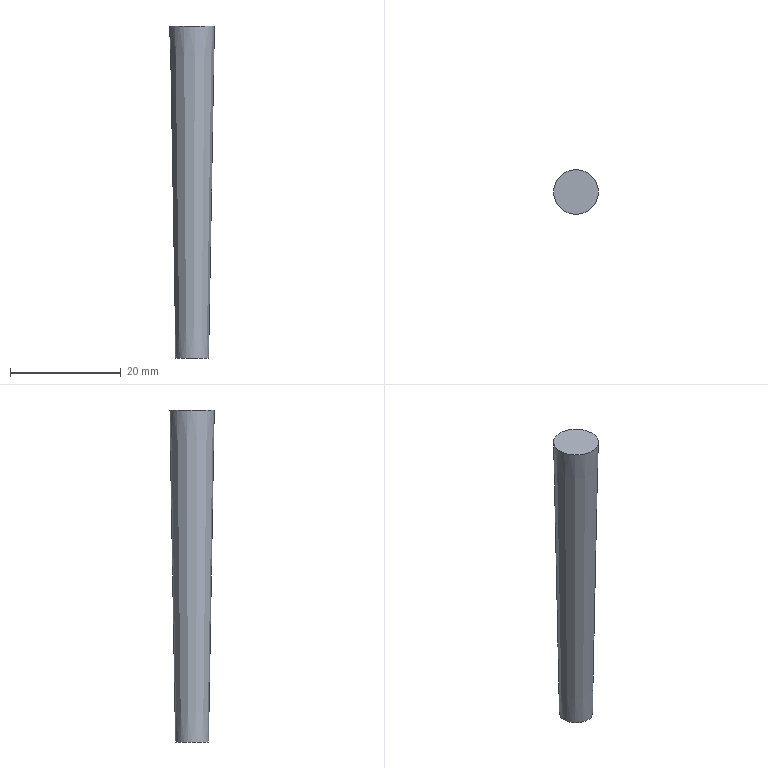Part | NX | features DATUM_CSYS 2, EXTRUDE 1, SKETCH 1 | 1 solid | 3 faces | box 8.095 x 8.095 x 60 mm | volume 2358 mm3 | plane 2 | cone 1
STEP:
#1=CARTESIAN_POINT('',(-4.047,0.,60.));
#2=VERTEX_POINT('',#1);
#3=CARTESIAN_POINT('',(0.,0.,60.));
#4=DIRECTION('',(0.,0.,-1.));
#5=DIRECTION('',(-1.,0.,0.));
#6=AXIS2_PLACEMENT_3D('',#3,#4,#5);
#7=CIRCLE('',#6,4.047);
#8=EDGE_CURVE('',#2,#2,#7,.T.);
#9=ORIENTED_EDGE('',*,*,#8,.T.);
#10=EDGE_LOOP('',(#9));
#11=FACE_BOUND('',#10,.T.);
#12=CARTESIAN_POINT('',(3.,0.,0.));
#13=VERTEX_POINT('',#12);
#14=CARTESIAN_POINT('',(0.,0.,0.));
#15=DIRECTION('',(0.,0.,-1.));
#16=DIRECTION('',(1.,0.,0.));
#17=AXIS2_PLACEMENT_3D('',#14,#15,#16);
#18=CIRCLE('',#17,3.);
#19=EDGE_CURVE('',#13,#13,#18,.T.);
#20=ORIENTED_EDGE('',*,*,#19,.F.);
#21=EDGE_LOOP('',(#20));
#22=FACE_BOUND('',#21,.T.);
#23=CARTESIAN_POINT('',(0.,0.,0.));
#24=DIRECTION('',(0.,0.,1.));
#25=DIRECTION('',(1.,0.,0.));
#26=AXIS2_PLACEMENT_3D('',#23,#24,#25);
#27=CONICAL_SURFACE('',#26,3.,0.01745);
#28=ADVANCED_FACE('',(#11,#22),#27,.T.);
#29=ORIENTED_EDGE('',*,*,#8,.F.);
#30=EDGE_LOOP('',(#29));
#31=FACE_BOUND('',#30,.T.);
#32=CARTESIAN_POINT('',(0.,0.,60.));
#33=DIRECTION('',(0.,0.,-1.));
#34=DIRECTION('',(-1.,0.,0.));
#35=AXIS2_PLACEMENT_3D('',#32,#33,#34);
#36=PLANE('',#35);
#37=ADVANCED_FACE('',(#31),#36,.F.);
#38=ORIENTED_EDGE('',*,*,#19,.T.);
#39=EDGE_LOOP('',(#38));
#40=FACE_BOUND('',#39,.T.);
#41=CARTESIAN_POINT('',(0.,0.,0.));
#42=DIRECTION('',(0.,0.,-1.));
#43=DIRECTION('',(-1.,0.,0.));
#44=AXIS2_PLACEMENT_3D('',#41,#42,#43);
#45=PLANE('',#44);
#46=ADVANCED_FACE('',(#40),#45,.T.);
#47=CLOSED_SHELL('',(#28,#37,#46));
#48=MANIFOLD_SOLID_BREP('',#47);
#49=(LENGTH_UNIT()NAMED_UNIT(*)SI_UNIT(.MILLI.,.METRE.));
#50=UNCERTAINTY_MEASURE_WITH_UNIT(LENGTH_MEASURE(0.00001),#49,'','');
#51=(NAMED_UNIT(*)PLANE_ANGLE_UNIT()SI_UNIT($,.RADIAN.));
#52=(NAMED_UNIT(*)SI_UNIT($,.STERADIAN.)SOLID_ANGLE_UNIT());
#53=(GEOMETRIC_REPRESENTATION_CONTEXT(3)GLOBAL_UNCERTAINTY_ASSIGNED_CONTEXT((#50))GLOBAL_UNIT_ASSIGNED_CONTEXT((#49,#51,#52))REPRESENTATION_CONTEXT('',''));
#54=ADVANCED_BREP_SHAPE_REPRESENTATION('',(#48),#53);